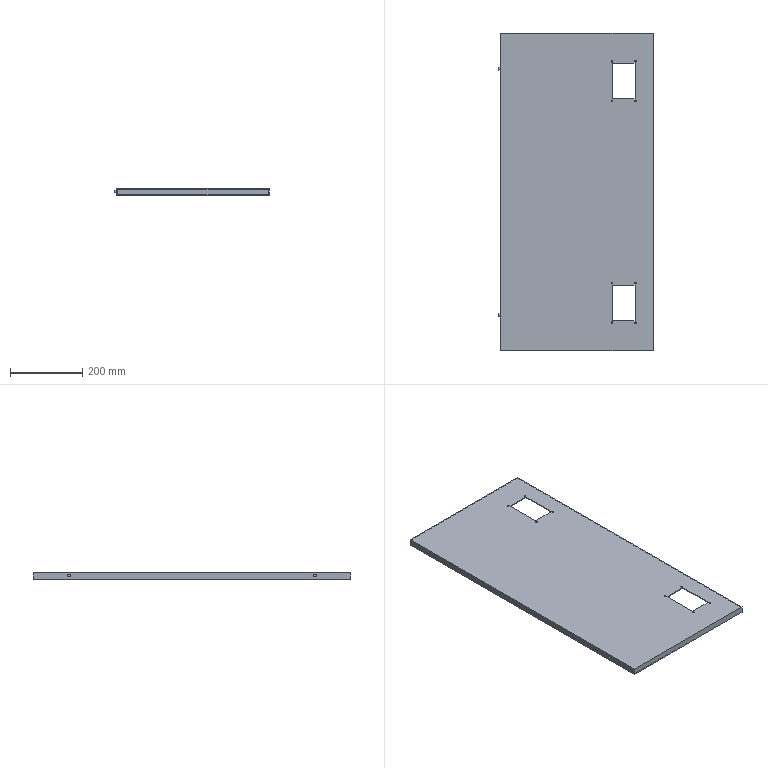Part | SolidWorks | features BaseBody 1 | 1 solid | 54 faces | box 426 x 876 x 18 mm | volume 861617 mm3 | cylinder 28 | plane 26 | commonest cylinder face diameters 5 x16 2.5 x8 8 x4